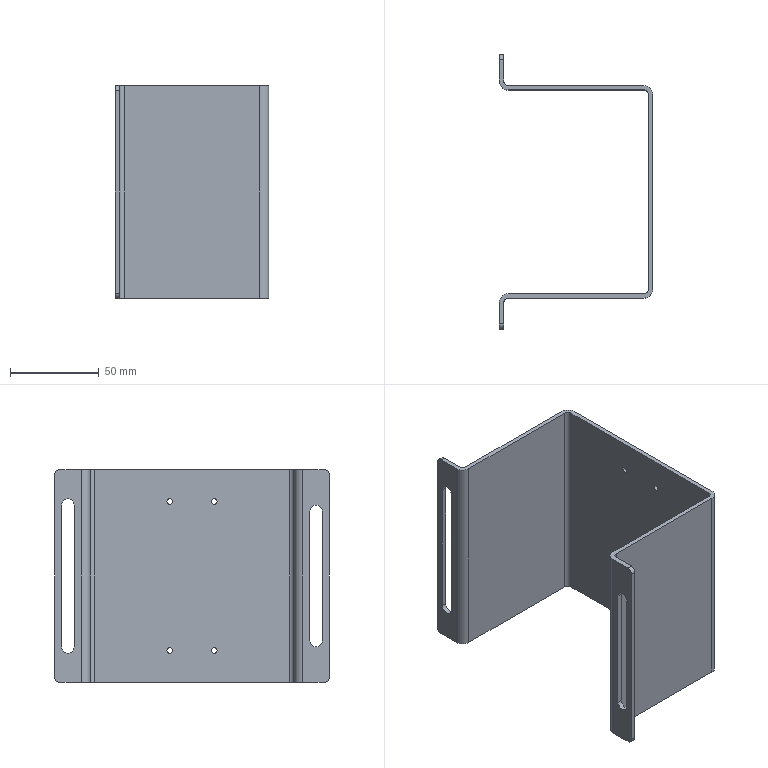Part | NX | features solid 2 | 1 solid | 50 faces | box 86.5 x 155 x 120 mm | volume 91997 mm3 | cylinder 32 | plane 18 | commonest cylinder face diameters 3.242 x16 5 x4 6 x4 7 x4 10 x4